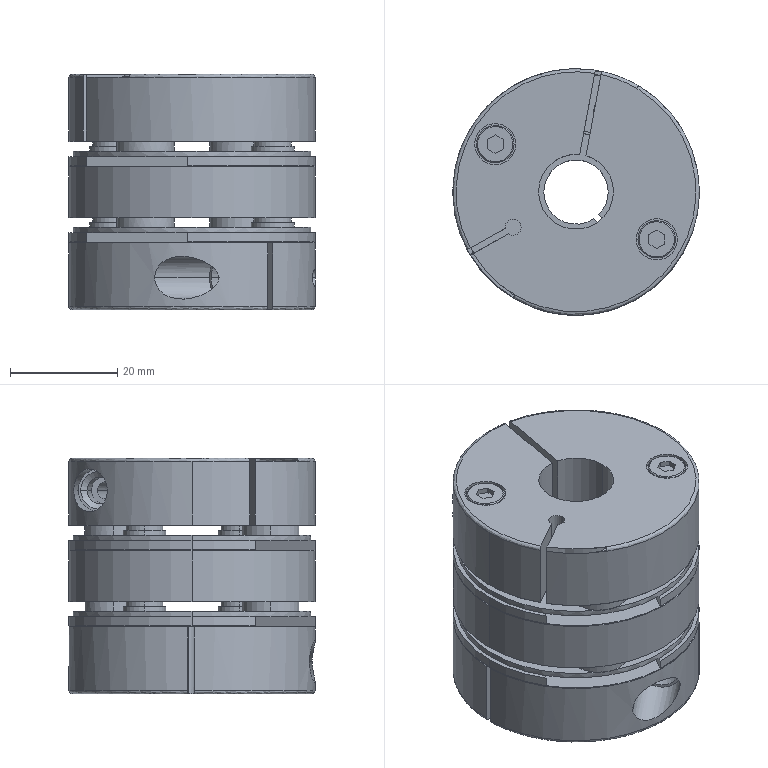Part | SolidWorks | features BaseBody 1 | 1 solid | 199 faces | box 46 x 46 x 44 mm | volume 54081 mm3 | cylinder 85 | plane 82 | cone 25 | spline 7 | commonest cylinder face diameters 7 x16 46 x13 8 x12 7.7 x8 10.7 x8 3 x4